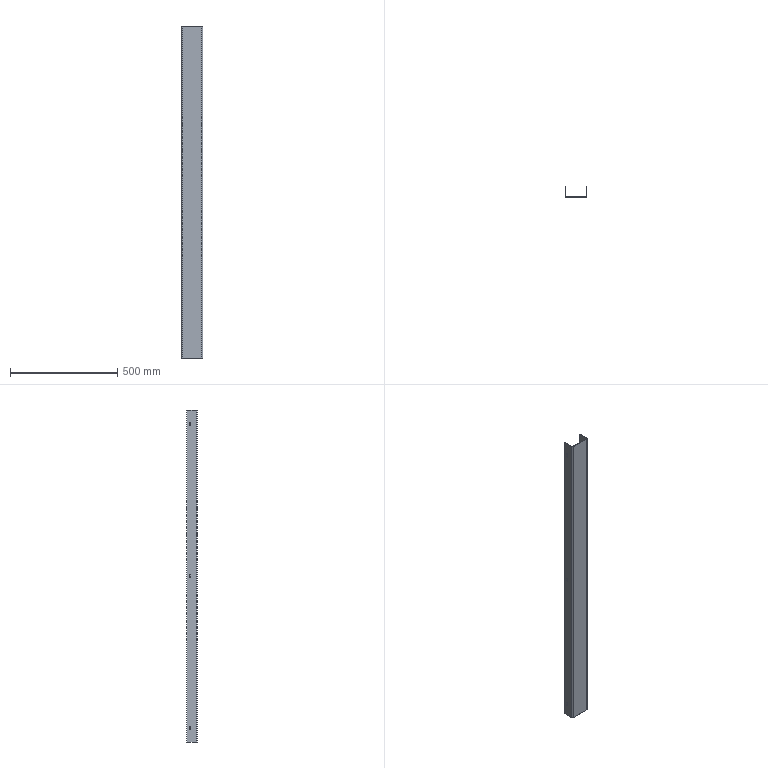Part | SolidWorks | features ICE 2, LPattern 2, FlatPattern 1, SMBaseFlange 1, SheetMetal 1 | 1 solid | 43 faces | box 100 x 50 x 1550 mm | volume 886864 mm3 | plane 24 | cylinder 19 | commonest cylinder face diameters 7 x9 6.4 x6 4 x2 10 x2
STEP:
#1=CARTESIAN_POINT('',(149.265,50.375,780.));
#2=VERTEX_POINT('',#1);
#3=CARTESIAN_POINT('',(149.265,46.875,783.5));
#4=VERTEX_POINT('',#3);
#5=CARTESIAN_POINT('',(149.265,46.875,780.));
#6=DIRECTION('',(1.,0.,0.));
#7=DIRECTION('',(0.,0.,-1.));
#8=AXIS2_PLACEMENT_3D('',#5,#6,#7);
#9=CIRCLE('',#8,3.5);
#10=EDGE_CURVE('',#2,#4,#9,.T.);
#11=ORIENTED_EDGE('',*,*,#10,.T.);
#12=CARTESIAN_POINT('',(146.265,46.875,783.5));
#13=VERTEX_POINT('',#12);
#14=CARTESIAN_POINT('',(156.265,46.875,783.5));
#15=DIRECTION('',(-1.,0.,0.));
#16=VECTOR('',#15,1000.);
#17=LINE('',#14,#16);
#18=EDGE_CURVE('',#4,#13,#17,.T.);
#19=ORIENTED_EDGE('',*,*,#18,.T.);
#20=CARTESIAN_POINT('',(146.265,50.375,780.));
#21=VERTEX_POINT('',#20);
#22=CARTESIAN_POINT('',(146.265,46.875,780.));
#23=DIRECTION('',(-1.,0.,0.));
#24=DIRECTION('',(0.,0.,1.));
#25=AXIS2_PLACEMENT_3D('',#22,#23,#24);
#26=CIRCLE('',#25,3.5);
#27=EDGE_CURVE('',#13,#21,#26,.T.);
#28=ORIENTED_EDGE('',*,*,#27,.T.);
#29=CARTESIAN_POINT('',(156.265,50.375,780.));
#30=DIRECTION('',(-1.,0.,0.));
#31=VECTOR('',#30,1000.);
#32=LINE('',#29,#31);
#33=EDGE_CURVE('',#2,#21,#32,.T.);
#34=ORIENTED_EDGE('',*,*,#33,.F.);
#35=EDGE_LOOP('',(#11,#19,#28,#34));
#36=FACE_OUTER_BOUND('',#35,.T.);
#37=CARTESIAN_POINT('',(156.265,46.875,780.));
#38=DIRECTION('',(-1.,0.,0.));
#39=DIRECTION('',(0.,0.,1.));
#40=AXIS2_PLACEMENT_3D('',#37,#38,#39);
#41=CYLINDRICAL_SURFACE('',#40,3.5);
#42=ADVANCED_FACE('',(#36),#41,.F.);
#43=CARTESIAN_POINT('',(149.265,50.375,70.));
#44=VERTEX_POINT('',#43);
#45=CARTESIAN_POINT('',(149.265,46.875,73.5));
#46=VERTEX_POINT('',#45);
#47=CARTESIAN_POINT('',(149.265,46.875,70.));
#48=DIRECTION('',(1.,0.,0.));
#49=DIRECTION('',(0.,0.,-1.));
#50=AXIS2_PLACEMENT_3D('',#47,#48,#49);
#51=CIRCLE('',#50,3.5);
#52=EDGE_CURVE('',#44,#46,#51,.T.);
#53=ORIENTED_EDGE('',*,*,#52,.T.);
#54=CARTESIAN_POINT('',(146.265,46.875,73.5));
#55=VERTEX_POINT('',#54);
#56=CARTESIAN_POINT('',(156.265,46.875,73.5));
#57=DIRECTION('',(-1.,0.,0.));
#58=VECTOR('',#57,1000.);
#59=LINE('',#56,#58);
#60=EDGE_CURVE('',#46,#55,#59,.T.);
#61=ORIENTED_EDGE('',*,*,#60,.T.);
#62=CARTESIAN_POINT('',(146.265,50.375,70.));
#63=VERTEX_POINT('',#62);
#64=CARTESIAN_POINT('',(146.265,46.875,70.));
#65=DIRECTION('',(-1.,0.,0.));
#66=DIRECTION('',(0.,0.,1.));
#67=AXIS2_PLACEMENT_3D('',#64,#65,#66);
#68=CIRCLE('',#67,3.5);
#69=EDGE_CURVE('',#55,#63,#68,.T.);
#70=ORIENTED_EDGE('',*,*,#69,.T.);
#71=CARTESIAN_POINT('',(156.265,50.375,70.));
#72=DIRECTION('',(-1.,0.,0.));
#73=VECTOR('',#72,1000.);
#74=LINE('',#71,#73);
#75=EDGE_CURVE('',#44,#63,#74,.T.);
#76=ORIENTED_EDGE('',*,*,#75,.F.);
#77=EDGE_LOOP('',(#53,#61,#70,#76));
#78=FACE_OUTER_BOUND('',#77,.T.);
#79=CARTESIAN_POINT('',(156.265,46.875,70.));
#80=DIRECTION('',(-1.,0.,0.));
#81=DIRECTION('',(0.,0.,1.));
#82=AXIS2_PLACEMENT_3D('',#79,#80,#81);
#83=CYLINDRICAL_SURFACE('',#82,3.5);
#84=ADVANCED_FACE('',(#78),#83,.F.);
#85=CARTESIAN_POINT('',(243.265,51.875,771.8));
#86=VERTEX_POINT('',#85);
#87=CARTESIAN_POINT('',(243.265,51.875,778.2));
#88=VERTEX_POINT('',#87);
#89=CARTESIAN_POINT('',(243.265,51.875,775.));
#90=DIRECTION('',(-1.,0.,0.));
#91=DIRECTION('',(0.,0.,1.));
#92=AXIS2_PLACEMENT_3D('',#89,#90,#91);
#93=CIRCLE('',#92,3.2);
#94=EDGE_CURVE('',#86,#88,#93,.T.);
#95=ORIENTED_EDGE('',*,*,#94,.T.);
#96=CARTESIAN_POINT('',(246.265,51.875,778.2));
#97=VERTEX_POINT('',#96);
#98=CARTESIAN_POINT('',(236.265,51.875,778.2));
#99=DIRECTION('',(1.,0.,0.));
#100=VECTOR('',#99,1000.);
#101=LINE('',#98,#100);
#102=EDGE_CURVE('',#88,#97,#101,.T.);
#103=ORIENTED_EDGE('',*,*,#102,.T.);
#104=CARTESIAN_POINT('',(246.265,51.875,771.8));
#105=VERTEX_POINT('',#104);
#106=CARTESIAN_POINT('',(246.265,51.875,775.));
#107=DIRECTION('',(1.,0.,0.));
#108=DIRECTION('',(0.,0.,-1.));
#109=AXIS2_PLACEMENT_3D('',#106,#107,#108);
#110=CIRCLE('',#109,3.2);
#111=EDGE_CURVE('',#97,#105,#110,.T.);
#112=ORIENTED_EDGE('',*,*,#111,.T.);
#113=CARTESIAN_POINT('',(236.265,51.875,771.8));
#114=DIRECTION('',(1.,0.,0.));
#115=VECTOR('',#114,1000.);
#116=LINE('',#113,#115);
#117=EDGE_CURVE('',#86,#105,#116,.T.);
#118=ORIENTED_EDGE('',*,*,#117,.F.);
#119=EDGE_LOOP('',(#95,#103,#112,#118));
#120=FACE_OUTER_BOUND('',#119,.T.);
#121=CARTESIAN_POINT('',(236.265,51.875,775.));
#122=DIRECTION('',(1.,0.,0.));
#123=DIRECTION('',(0.,0.,-1.));
#124=AXIS2_PLACEMENT_3D('',#121,#122,#123);
#125=CYLINDRICAL_SURFACE('',#124,3.2);
#126=ADVANCED_FACE('',(#120),#125,.F.);
#127=CARTESIAN_POINT('',(243.265,51.875,1484.3));
#128=VERTEX_POINT('',#127);
#129=CARTESIAN_POINT('',(243.265,51.875,1490.7));
#130=VERTEX_POINT('',#129);
#131=CARTESIAN_POINT('',(243.265,51.875,1487.5));
#132=DIRECTION('',(-1.,0.,0.));
#133=DIRECTION('',(0.,0.,1.));
#134=AXIS2_PLACEMENT_3D('',#131,#132,#133);
#135=CIRCLE('',#134,3.2);
#136=EDGE_CURVE('',#128,#130,#135,.T.);
#137=ORIENTED_EDGE('',*,*,#136,.T.);
#138=CARTESIAN_POINT('',(246.265,51.875,1490.7));
#139=VERTEX_POINT('',#138);
#140=CARTESIAN_POINT('',(236.265,51.875,1490.7));
#141=DIRECTION('',(1.,0.,0.));
#142=VECTOR('',#141,1000.);
#143=LINE('',#140,#142);
#144=EDGE_CURVE('',#130,#139,#143,.T.);
#145=ORIENTED_EDGE('',*,*,#144,.T.);
#146=CARTESIAN_POINT('',(246.265,51.875,1484.3));
#147=VERTEX_POINT('',#146);
#148=CARTESIAN_POINT('',(246.265,51.875,1487.5));
#149=DIRECTION('',(1.,0.,0.));
#150=DIRECTION('',(0.,0.,-1.));
#151=AXIS2_PLACEMENT_3D('',#148,#149,#150);
#152=CIRCLE('',#151,3.2);
#153=EDGE_CURVE('',#139,#147,#152,.T.);
#154=ORIENTED_EDGE('',*,*,#153,.T.);
#155=CARTESIAN_POINT('',(236.265,51.875,1484.3));
#156=DIRECTION('',(1.,0.,0.));
#157=VECTOR('',#156,1000.);
#158=LINE('',#155,#157);
#159=EDGE_CURVE('',#128,#147,#158,.T.);
#160=ORIENTED_EDGE('',*,*,#159,.F.);
#161=EDGE_LOOP('',(#137,#145,#154,#160));
#162=FACE_OUTER_BOUND('',#161,.T.);
#163=CARTESIAN_POINT('',(236.265,51.875,1487.5));
#164=DIRECTION('',(1.,0.,0.));
#165=DIRECTION('',(0.,0.,-1.));
#166=AXIS2_PLACEMENT_3D('',#163,#164,#165);
#167=CYLINDRICAL_SURFACE('',#166,3.2);
#168=ADVANCED_FACE('',(#162),#167,.F.);
#169=CARTESIAN_POINT('',(243.265,51.875,59.3));
#170=VERTEX_POINT('',#169);
#171=CARTESIAN_POINT('',(243.265,51.875,65.7));
#172=VERTEX_POINT('',#171);
#173=CARTESIAN_POINT('',(243.265,51.875,62.5));
#174=DIRECTION('',(-1.,0.,0.));
#175=DIRECTION('',(0.,0.,1.));
#176=AXIS2_PLACEMENT_3D('',#173,#174,#175);
#177=CIRCLE('',#176,3.2);
#178=EDGE_CURVE('',#170,#172,#177,.T.);
#179=ORIENTED_EDGE('',*,*,#178,.T.);
#180=CARTESIAN_POINT('',(246.265,51.875,65.7));
#181=VERTEX_POINT('',#180);
#182=CARTESIAN_POINT('',(236.265,51.875,65.7));
#183=DIRECTION('',(1.,0.,0.));
#184=VECTOR('',#183,1000.);
#185=LINE('',#182,#184);
#186=EDGE_CURVE('',#172,#181,#185,.T.);
#187=ORIENTED_EDGE('',*,*,#186,.T.);
#188=CARTESIAN_POINT('',(246.265,51.875,59.3));
#189=VERTEX_POINT('',#188);
#190=CARTESIAN_POINT('',(246.265,51.875,62.5));
#191=DIRECTION('',(1.,0.,0.));
#192=DIRECTION('',(0.,0.,-1.));
#193=AXIS2_PLACEMENT_3D('',#190,#191,#192);
#194=CIRCLE('',#193,3.2);
#195=EDGE_CURVE('',#181,#189,#194,.T.);
#196=ORIENTED_EDGE('',*,*,#195,.T.);
#197=CARTESIAN_POINT('',(236.265,51.875,59.3));
#198=DIRECTION('',(1.,0.,0.));
#199=VECTOR('',#198,1000.);
#200=LINE('',#197,#199);
#201=EDGE_CURVE('',#170,#189,#200,.T.);
#202=ORIENTED_EDGE('',*,*,#201,.F.);
#203=EDGE_LOOP('',(#179,#187,#196,#202));
#204=FACE_OUTER_BOUND('',#203,.T.);
#205=CARTESIAN_POINT('',(236.265,51.875,62.5));
#206=DIRECTION('',(1.,0.,0.));
#207=DIRECTION('',(0.,0.,-1.));
#208=AXIS2_PLACEMENT_3D('',#205,#206,#207);
#209=CYLINDRICAL_SURFACE('',#208,3.2);
#210=ADVANCED_FACE('',(#204),#209,.F.);
#211=CARTESIAN_POINT('',(149.265,50.375,1490.));
#212=VERTEX_POINT('',#211);
#213=CARTESIAN_POINT('',(149.265,46.875,1493.5));
#214=VERTEX_POINT('',#213);
#215=CARTESIAN_POINT('',(149.265,46.875,1490.));
#216=DIRECTION('',(1.,0.,0.));
#217=DIRECTION('',(0.,0.,-1.));
#218=AXIS2_PLACEMENT_3D('',#215,#216,#217);
#219=CIRCLE('',#218,3.5);
#220=EDGE_CURVE('',#212,#214,#219,.T.);
#221=ORIENTED_EDGE('',*,*,#220,.T.);
#222=CARTESIAN_POINT('',(146.265,46.875,1493.5));
#223=VERTEX_POINT('',#222);
#224=CARTESIAN_POINT('',(156.265,46.875,1493.5));
#225=DIRECTION('',(-1.,0.,0.));
#226=VECTOR('',#225,1000.);
#227=LINE('',#224,#226);
#228=EDGE_CURVE('',#214,#223,#227,.T.);
#229=ORIENTED_EDGE('',*,*,#228,.T.);
#230=CARTESIAN_POINT('',(146.265,50.375,1490.));
#231=VERTEX_POINT('',#230);
#232=CARTESIAN_POINT('',(146.265,46.875,1490.));
#233=DIRECTION('',(-1.,0.,0.));
#234=DIRECTION('',(0.,0.,1.));
#235=AXIS2_PLACEMENT_3D('',#232,#233,#234);
#236=CIRCLE('',#235,3.5);
#237=EDGE_CURVE('',#223,#231,#236,.T.);
#238=ORIENTED_EDGE('',*,*,#237,.T.);
#239=CARTESIAN_POINT('',(156.265,50.375,1490.));
#240=DIRECTION('',(-1.,0.,0.));
#241=VECTOR('',#240,1000.);
#242=LINE('',#239,#241);
#243=EDGE_CURVE('',#212,#231,#242,.T.);
#244=ORIENTED_EDGE('',*,*,#243,.F.);
#245=EDGE_LOOP('',(#221,#229,#238,#244));
#246=FACE_OUTER_BOUND('',#245,.T.);
#247=CARTESIAN_POINT('',(156.265,46.875,1490.));
#248=DIRECTION('',(-1.,0.,0.));
#249=DIRECTION('',(0.,0.,1.));
#250=AXIS2_PLACEMENT_3D('',#247,#248,#249);
#251=CYLINDRICAL_SURFACE('',#250,3.5);
#252=ADVANCED_FACE('',(#246),#251,.F.);
#253=CARTESIAN_POINT('',(149.265,43.375,1490.));
#254=VERTEX_POINT('',#253);
#255=CARTESIAN_POINT('',(149.265,43.375,1480.));
#256=VERTEX_POINT('',#255);
#257=CARTESIAN_POINT('',(149.265,43.375,2970.));
#258=DIRECTION('',(0.,0.,-1.));
#259=VECTOR('',#258,1000.);
#260=LINE('',#257,#259);
#261=EDGE_CURVE('',#254,#256,#260,.T.);
#262=ORIENTED_EDGE('',*,*,#261,.T.);
#263=CARTESIAN_POINT('',(146.265,43.375,1480.));
#264=VERTEX_POINT('',#263);
#265=CARTESIAN_POINT('',(156.265,43.375,1480.));
#266=DIRECTION('',(-1.,0.,0.));
#267=VECTOR('',#266,1000.);
#268=LINE('',#265,#267);
#269=EDGE_CURVE('',#256,#264,#268,.T.);
#270=ORIENTED_EDGE('',*,*,#269,.T.);
#271=CARTESIAN_POINT('',(146.265,43.375,1490.));
#272=VERTEX_POINT('',#271);
#273=CARTESIAN_POINT('',(146.265,43.375,1480.));
#274=DIRECTION('',(0.,0.,1.));
#275=VECTOR('',#274,1000.);
#276=LINE('',#273,#275);
#277=EDGE_CURVE('',#264,#272,#276,.T.);
#278=ORIENTED_EDGE('',*,*,#277,.T.);
#279=CARTESIAN_POINT('',(156.265,43.375,1490.));
#280=DIRECTION('',(-1.,0.,0.));
#281=VECTOR('',#280,1000.);
#282=LINE('',#279,#281);
#283=EDGE_CURVE('',#254,#272,#282,.T.);
#284=ORIENTED_EDGE('',*,*,#283,.F.);
#285=EDGE_LOOP('',(#262,#270,#278,#284));
#286=FACE_OUTER_BOUND('',#285,.T.);
#287=CARTESIAN_POINT('',(156.265,43.375,1480.));
#288=DIRECTION('',(0.,-1.,0.));
#289=DIRECTION('',(0.,0.,-1.));
#290=AXIS2_PLACEMENT_3D('',#287,#288,#289);
#291=PLANE('',#290);
#292=ADVANCED_FACE('',(#286),#291,.F.);
#293=ORIENTED_EDGE('',*,*,#228,.F.);
#294=CARTESIAN_POINT('',(149.265,46.875,1490.));
#295=DIRECTION('',(1.,0.,0.));
#296=DIRECTION('',(0.,0.,-1.));
#297=AXIS2_PLACEMENT_3D('',#294,#295,#296);
#298=CIRCLE('',#297,3.5);
#299=EDGE_CURVE('',#214,#254,#298,.T.);
#300=ORIENTED_EDGE('',*,*,#299,.T.);
#301=ORIENTED_EDGE('',*,*,#283,.T.);
#302=CARTESIAN_POINT('',(146.265,46.875,1490.));
#303=DIRECTION('',(-1.,0.,0.));
#304=DIRECTION('',(0.,0.,1.));
#305=AXIS2_PLACEMENT_3D('',#302,#303,#304);
#306=CIRCLE('',#305,3.5);
#307=EDGE_CURVE('',#272,#223,#306,.T.);
#308=ORIENTED_EDGE('',*,*,#307,.T.);
#309=EDGE_LOOP('',(#293,#300,#301,#308));
#310=FACE_OUTER_BOUND('',#309,.T.);
#311=CARTESIAN_POINT('',(156.265,46.875,1490.));
#312=DIRECTION('',(-1.,0.,0.));
#313=DIRECTION('',(0.,0.,1.));
#314=AXIS2_PLACEMENT_3D('',#311,#312,#313);
#315=CYLINDRICAL_SURFACE('',#314,3.5);
#316=ADVANCED_FACE('',(#310),#315,.F.);
#317=CARTESIAN_POINT('',(149.265,50.375,1480.));
#318=VERTEX_POINT('',#317);
#319=CARTESIAN_POINT('',(149.265,50.375,2970.));
#320=DIRECTION('',(0.,0.,1.));
#321=VECTOR('',#320,1000.);
#322=LINE('',#319,#321);
#323=EDGE_CURVE('',#318,#212,#322,.T.);
#324=ORIENTED_EDGE('',*,*,#323,.T.);
#325=ORIENTED_EDGE('',*,*,#243,.T.);
#326=CARTESIAN_POINT('',(146.265,50.375,1480.));
#327=VERTEX_POINT('',#326);
#328=CARTESIAN_POINT('',(146.265,50.375,1480.));
#329=DIRECTION('',(0.,0.,-1.));
#330=VECTOR('',#329,1000.);
#331=LINE('',#328,#330);
#332=EDGE_CURVE('',#231,#327,#331,.T.);
#333=ORIENTED_EDGE('',*,*,#332,.T.);
#334=CARTESIAN_POINT('',(156.265,50.375,1480.));
#335=DIRECTION('',(-1.,0.,0.));
#336=VECTOR('',#335,1000.);
#337=LINE('',#334,#336);
#338=EDGE_CURVE('',#318,#327,#337,.T.);
#339=ORIENTED_EDGE('',*,*,#338,.F.);
#340=EDGE_LOOP('',(#324,#325,#333,#339));
#341=FACE_OUTER_BOUND('',#340,.T.);
#342=CARTESIAN_POINT('',(156.265,50.375,1480.));
#343=DIRECTION('',(0.,1.,0.));
#344=DIRECTION('',(0.,0.,1.));
#345=AXIS2_PLACEMENT_3D('',#342,#343,#344);
#346=PLANE('',#345);
#347=ADVANCED_FACE('',(#341),#346,.F.);
#348=CARTESIAN_POINT('',(149.265,46.875,1480.));
#349=DIRECTION('',(1.,0.,0.));
#350=DIRECTION('',(0.,0.,-1.));
#351=AXIS2_PLACEMENT_3D('',#348,#349,#350);
#352=CIRCLE('',#351,3.5);
#353=EDGE_CURVE('',#256,#318,#352,.T.);
#354=ORIENTED_EDGE('',*,*,#353,.T.);
#355=ORIENTED_EDGE('',*,*,#338,.T.);
#356=CARTESIAN_POINT('',(146.265,46.875,1480.));
#357=DIRECTION('',(-1.,0.,0.));
#358=DIRECTION('',(0.,0.,1.));
#359=AXIS2_PLACEMENT_3D('',#356,#357,#358);
#360=CIRCLE('',#359,3.5);
#361=EDGE_CURVE('',#327,#264,#360,.T.);
#362=ORIENTED_EDGE('',*,*,#361,.T.);
#363=ORIENTED_EDGE('',*,*,#269,.F.);
#364=EDGE_LOOP('',(#354,#355,#362,#363));
#365=FACE_OUTER_BOUND('',#364,.T.);
#366=CARTESIAN_POINT('',(156.265,46.875,1480.));
#367=DIRECTION('',(-1.,0.,0.));
#368=DIRECTION('',(0.,0.,1.));
#369=AXIS2_PLACEMENT_3D('',#366,#367,#368);
#370=CYLINDRICAL_SURFACE('',#369,3.5);
#371=ADVANCED_FACE('',(#365),#370,.F.);
#372=ORIENTED_EDGE('',*,*,#186,.F.);
#373=CARTESIAN_POINT('',(243.265,51.875,62.5));
#374=DIRECTION('',(-1.,0.,0.));
#375=DIRECTION('',(0.,0.,1.));
#376=AXIS2_PLACEMENT_3D('',#373,#374,#375);
#377=CIRCLE('',#376,3.2);
#378=EDGE_CURVE('',#172,#170,#377,.T.);
#379=ORIENTED_EDGE('',*,*,#378,.T.);
#380=ORIENTED_EDGE('',*,*,#201,.T.);
#381=CARTESIAN_POINT('',(246.265,51.875,62.5));
#382=DIRECTION('',(1.,0.,0.));
#383=DIRECTION('',(0.,0.,-1.));
#384=AXIS2_PLACEMENT_3D('',#381,#382,#383);
#385=CIRCLE('',#384,3.2);
#386=EDGE_CURVE('',#189,#181,#385,.T.);
#387=ORIENTED_EDGE('',*,*,#386,.T.);
#388=EDGE_LOOP('',(#372,#379,#380,#387));
#389=FACE_OUTER_BOUND('',#388,.T.);
#390=CARTESIAN_POINT('',(236.265,51.875,62.5));
#391=DIRECTION('',(1.,0.,0.));
#392=DIRECTION('',(0.,0.,-1.));
#393=AXIS2_PLACEMENT_3D('',#390,#391,#392);
#394=CYLINDRICAL_SURFACE('',#393,3.2);
#395=ADVANCED_FACE('',(#389),#394,.F.);
#396=CARTESIAN_POINT('',(146.265,16.875,1550.));
#397=VERTEX_POINT('',#396);
#398=CARTESIAN_POINT('',(149.265,16.875,1550.));
#399=VERTEX_POINT('',#398);
#400=CARTESIAN_POINT('',(146.265,16.875,1550.));
#401=DIRECTION('',(1.,0.,0.));
#402=VECTOR('',#401,1000.);
#403=LINE('',#400,#402);
#404=EDGE_CURVE('',#397,#399,#403,.T.);
#405=ORIENTED_EDGE('',*,*,#404,.F.);
#406=CARTESIAN_POINT('',(151.265,11.875,1550.));
#407=VERTEX_POINT('',#406);
#408=CARTESIAN_POINT('',(151.265,16.875,1550.));
#409=DIRECTION('',(0.,0.,1.));
#410=DIRECTION('',(-1.,0.,0.));
#411=AXIS2_PLACEMENT_3D('',#408,#409,#410);
#412=CIRCLE('',#411,5.);
#413=EDGE_CURVE('',#397,#407,#412,.T.);
#414=ORIENTED_EDGE('',*,*,#413,.T.);
#415=CARTESIAN_POINT('',(151.265,14.875,1550.));
#416=VERTEX_POINT('',#415);
#417=CARTESIAN_POINT('',(151.265,14.875,1550.));
#418=DIRECTION('',(0.,-1.,0.));
#419=VECTOR('',#418,1000.);
#420=LINE('',#417,#419);
#421=EDGE_CURVE('',#416,#407,#420,.T.);
#422=ORIENTED_EDGE('',*,*,#421,.F.);
#423=CARTESIAN_POINT('',(151.265,16.875,1550.));
#424=DIRECTION('',(0.,0.,1.));
#425=DIRECTION('',(1.,0.,0.));
#426=AXIS2_PLACEMENT_3D('',#423,#424,#425);
#427=CIRCLE('',#426,2.);
#428=EDGE_CURVE('',#399,#416,#427,.T.);
#429=ORIENTED_EDGE('',*,*,#428,.F.);
#430=EDGE_LOOP('',(#405,#414,#422,#429));
#431=FACE_OUTER_BOUND('',#430,.T.);
#432=CARTESIAN_POINT('',(146.265,16.875,1550.));
#433=DIRECTION('',(0.,0.,1.));
#434=DIRECTION('',(1.,0.,0.));
#435=AXIS2_PLACEMENT_3D('',#432,#433,#434);
#436=PLANE('',#435);
#437=ADVANCED_FACE('',(#431),#436,.T.);
#438=CARTESIAN_POINT('',(146.265,61.875,1550.));
#439=VERTEX_POINT('',#438);
#440=CARTESIAN_POINT('',(146.265,61.875,1550.));
#441=DIRECTION('',(0.,-1.,0.));
#442=VECTOR('',#441,1000.);
#443=LINE('',#440,#442);
#444=EDGE_CURVE('',#439,#397,#443,.T.);
#445=ORIENTED_EDGE('',*,*,#444,.T.);
#446=ORIENTED_EDGE('',*,*,#404,.T.);
#447=CARTESIAN_POINT('',(149.265,61.875,1550.));
#448=VERTEX_POINT('',#447);
#449=CARTESIAN_POINT('',(149.265,61.875,1550.));
#450=DIRECTION('',(0.,-1.,0.));
#451=VECTOR('',#450,1000.);
#452=LINE('',#449,#451);
#453=EDGE_CURVE('',#448,#399,#452,.T.);
#454=ORIENTED_EDGE('',*,*,#453,.F.);
#455=CARTESIAN_POINT('',(146.265,61.875,1550.));
#456=DIRECTION('',(1.,0.,0.));
#457=VECTOR('',#456,1000.);
#458=LINE('',#455,#457);
#459=EDGE_CURVE('',#439,#448,#458,.T.);
#460=ORIENTED_EDGE('',*,*,#459,.F.);
#461=EDGE_LOOP('',(#445,#446,#454,#460));
#462=FACE_OUTER_BOUND('',#461,.T.);
#463=CARTESIAN_POINT('',(151.265,14.875,1550.));
#464=DIRECTION('',(0.,0.,1.));
#465=DIRECTION('',(1.,0.,0.));
#466=AXIS2_PLACEMENT_3D('',#463,#464,#465);
#467=PLANE('',#466);
#468=ADVANCED_FACE('',(#462),#467,.T.);
#469=CARTESIAN_POINT('',(151.265,11.875,0.));
#470=VERTEX_POINT('',#469);
#471=CARTESIAN_POINT('',(151.265,14.875,0.));
#472=VERTEX_POINT('',#471);
#473=CARTESIAN_POINT('',(151.265,11.875,0.));
#474=DIRECTION('',(0.,1.,0.));
#475=VECTOR('',#474,1000.);
#476=LINE('',#473,#475);
#477=EDGE_CURVE('',#470,#472,#476,.T.);
#478=ORIENTED_EDGE('',*,*,#477,.F.);
#479=CARTESIAN_POINT('',(146.265,16.875,0.));
#480=VERTEX_POINT('',#479);
#481=CARTESIAN_POINT('',(151.265,16.875,0.));
#482=DIRECTION('',(0.,0.,1.));
#483=DIRECTION('',(-1.,0.,0.));
#484=AXIS2_PLACEMENT_3D('',#481,#482,#483);
#485=CIRCLE('',#484,5.);
#486=EDGE_CURVE('',#480,#470,#485,.T.);
#487=ORIENTED_EDGE('',*,*,#486,.F.);
#488=CARTESIAN_POINT('',(149.265,16.875,0.));
#489=VERTEX_POINT('',#488);
#490=CARTESIAN_POINT('',(149.265,16.875,0.));
#491=DIRECTION('',(-1.,0.,0.));
#492=VECTOR('',#491,1000.);
#493=LINE('',#490,#492);
#494=EDGE_CURVE('',#489,#480,#493,.T.);
#495=ORIENTED_EDGE('',*,*,#494,.F.);
#496=CARTESIAN_POINT('',(151.265,16.875,0.));
#497=DIRECTION('',(0.,0.,1.));
#498=DIRECTION('',(1.,0.,0.));
#499=AXIS2_PLACEMENT_3D('',#496,#497,#498);
#500=CIRCLE('',#499,2.);
#501=EDGE_CURVE('',#489,#472,#500,.T.);
#502=ORIENTED_EDGE('',*,*,#501,.T.);
#503=EDGE_LOOP('',(#478,#487,#495,#502));
#504=FACE_OUTER_BOUND('',#503,.T.);
#505=CARTESIAN_POINT('',(151.265,11.875,0.));
#506=DIRECTION('',(0.,0.,-1.));
#507=DIRECTION('',(-1.,0.,0.));
#508=AXIS2_PLACEMENT_3D('',#505,#506,#507);
#509=PLANE('',#508);
#510=ADVANCED_FACE('',(#504),#509,.T.);
#511=CARTESIAN_POINT('',(241.265,11.875,0.));
#512=VERTEX_POINT('',#511);
#513=CARTESIAN_POINT('',(146.265,11.875,0.));
#514=DIRECTION('',(1.,0.,0.));
#515=VECTOR('',#514,1000.);
#516=LINE('',#513,#515);
#517=EDGE_CURVE('',#470,#512,#516,.T.);
#518=ORIENTED_EDGE('',*,*,#517,.F.);
#519=ORIENTED_EDGE('',*,*,#477,.T.);
#520=CARTESIAN_POINT('',(241.265,14.875,0.));
#521=VERTEX_POINT('',#520);
#522=CARTESIAN_POINT('',(146.265,14.875,0.));
#523=DIRECTION('',(1.,0.,0.));
#524=VECTOR('',#523,1000.);
#525=LINE('',#522,#524);
#526=EDGE_CURVE('',#472,#521,#525,.T.);
#527=ORIENTED_EDGE('',*,*,#526,.T.);
#528=CARTESIAN_POINT('',(241.265,14.875,0.));
#529=DIRECTION('',(0.,-1.,0.));
#530=VECTOR('',#529,1000.);
#531=LINE('',#528,#530);
#532=EDGE_CURVE('',#521,#512,#531,.T.);
#533=ORIENTED_EDGE('',*,*,#532,.T.);
#534=EDGE_LOOP('',(#518,#519,#527,#533));
#535=FACE_OUTER_BOUND('',#534,.T.);
#536=CARTESIAN_POINT('',(149.265,16.875,0.));
#537=DIRECTION('',(0.,0.,-1.));
#538=DIRECTION('',(-1.,0.,0.));
#539=AXIS2_PLACEMENT_3D('',#536,#537,#538);
#540=PLANE('',#539);
#541=ADVANCED_FACE('',(#535),#540,.T.);
#542=CARTESIAN_POINT('',(241.265,11.875,1550.));
#543=VERTEX_POINT('',#542);
#544=CARTESIAN_POINT('',(241.265,14.875,1550.));
#545=VERTEX_POINT('',#544);
#546=CARTESIAN_POINT('',(241.265,11.875,1550.));
#547=DIRECTION('',(0.,1.,0.));
#548=VECTOR('',#547,1000.);
#549=LINE('',#546,#548);
#550=EDGE_CURVE('',#543,#545,#549,.T.);
#551=ORIENTED_EDGE('',*,*,#550,.F.);
#552=CARTESIAN_POINT('',(246.265,16.875,1550.));
#553=VERTEX_POINT('',#552);
#554=CARTESIAN_POINT('',(241.265,16.875,1550.));
#555=DIRECTION('',(0.,0.,1.));
#556=DIRECTION('',(-1.,0.,0.));
#557=AXIS2_PLACEMENT_3D('',#554,#555,#556);
#558=CIRCLE('',#557,5.);
#559=EDGE_CURVE('',#543,#553,#558,.T.);
#560=ORIENTED_EDGE('',*,*,#559,.T.);
#561=CARTESIAN_POINT('',(243.265,16.875,1550.));
#562=VERTEX_POINT('',#561);
#563=CARTESIAN_POINT('',(243.265,16.875,1550.));
#564=DIRECTION('',(1.,0.,0.));
#565=VECTOR('',#564,1000.);
#566=LINE('',#563,#565);
#567=EDGE_CURVE('',#562,#553,#566,.T.);
#568=ORIENTED_EDGE('',*,*,#567,.F.);
#569=CARTESIAN_POINT('',(241.265,16.875,1550.));
#570=DIRECTION('',(0.,0.,1.));
#571=DIRECTION('',(1.,0.,0.));
#572=AXIS2_PLACEMENT_3D('',#569,#570,#571);
#573=CIRCLE('',#572,2.);
#574=EDGE_CURVE('',#545,#562,#573,.T.);
#575=ORIENTED_EDGE('',*,*,#574,.F.);
#576=EDGE_LOOP('',(#551,#560,#568,#575));
#577=FACE_OUTER_BOUND('',#576,.T.);
#578=CARTESIAN_POINT('',(241.265,11.875,1550.));
#579=DIRECTION('',(0.,0.,1.));
#580=DIRECTION('',(1.,0.,0.));
#581=AXIS2_PLACEMENT_3D('',#578,#579,#580);
#582=PLANE('',#581);
#583=ADVANCED_FACE('',(#577),#582,.T.);
#584=CARTESIAN_POINT('',(146.265,11.875,1550.));
#585=DIRECTION('',(1.,0.,0.));
#586=VECTOR('',#585,1000.);
#587=LINE('',#584,#586);
#588=EDGE_CURVE('',#407,#543,#587,.T.);
#589=ORIENTED_EDGE('',*,*,#588,.T.);
#590=ORIENTED_EDGE('',*,*,#550,.T.);
#591=CARTESIAN_POINT('',(146.265,14.875,1550.));
#592=DIRECTION('',(1.,0.,0.));
#593=VECTOR('',#592,1000.);
#594=LINE('',#591,#593);
#595=EDGE_CURVE('',#416,#545,#594,.T.);
#596=ORIENTED_EDGE('',*,*,#595,.F.);
#597=ORIENTED_EDGE('',*,*,#421,.T.);
#598=EDGE_LOOP('',(#589,#590,#596,#597));
#599=FACE_OUTER_BOUND('',#598,.T.);
#600=CARTESIAN_POINT('',(243.265,16.875,1550.));
#601=DIRECTION('',(0.,0.,1.));
#602=DIRECTION('',(1.,0.,0.));
#603=AXIS2_PLACEMENT_3D('',#600,#601,#602);
#604=PLANE('',#603);
#605=ADVANCED_FACE('',(#599),#604,.T.);
#606=CARTESIAN_POINT('',(246.265,16.875,0.));
#607=VERTEX_POINT('',#606);
#608=CARTESIAN_POINT('',(243.265,16.875,0.));
#609=VERTEX_POINT('',#608);
#610=CARTESIAN_POINT('',(246.265,16.875,0.));
#611=DIRECTION('',(-1.,0.,0.));
#612=VECTOR('',#611,1000.);
#613=LINE('',#610,#612);
#614=EDGE_CURVE('',#607,#609,#613,.T.);
#615=ORIENTED_EDGE('',*,*,#614,.F.);
#616=CARTESIAN_POINT('',(241.265,16.875,0.));
#617=DIRECTION('',(0.,0.,1.));
#618=DIRECTION('',(-1.,0.,0.));
#619=AXIS2_PLACEMENT_3D('',#616,#617,#618);
#620=CIRCLE('',#619,5.);
#621=EDGE_CURVE('',#512,#607,#620,.T.);
#622=ORIENTED_EDGE('',*,*,#621,.F.);
#623=ORIENTED_EDGE('',*,*,#532,.F.);
#624=CARTESIAN_POINT('',(241.265,16.875,0.));
#625=DIRECTION('',(0.,0.,1.));
#626=DIRECTION('',(1.,0.,0.));
#627=AXIS2_PLACEMENT_3D('',#624,#625,#626);
#628=CIRCLE('',#627,2.);
#629=EDGE_CURVE('',#521,#609,#628,.T.);
#630=ORIENTED_EDGE('',*,*,#629,.T.);
#631=EDGE_LOOP('',(#615,#622,#623,#630));
#632=FACE_OUTER_BOUND('',#631,.T.);
#633=CARTESIAN_POINT('',(246.265,16.875,0.));
#634=DIRECTION('',(0.,0.,-1.));
#635=DIRECTION('',(-1.,0.,0.));
#636=AXIS2_PLACEMENT_3D('',#633,#634,#635);
#637=PLANE('',#636);
#638=ADVANCED_FACE('',(#632),#637,.T.);
#639=CARTESIAN_POINT('',(246.265,61.875,0.));
#640=VERTEX_POINT('',#639);
#641=CARTESIAN_POINT('',(246.265,11.875,0.));
#642=DIRECTION('',(0.,1.,0.));
#643=VECTOR('',#642,1000.);
#644=LINE('',#641,#643);
#645=EDGE_CURVE('',#607,#640,#644,.T.);
#646=ORIENTED_EDGE('',*,*,#645,.F.);
#647=ORIENTED_EDGE('',*,*,#614,.T.);
#648=CARTESIAN_POINT('',(243.265,61.875,0.));
#649=VERTEX_POINT('',#648);
#650=CARTESIAN_POINT('',(243.265,11.875,0.));
#651=DIRECTION('',(0.,1.,0.));
#652=VECTOR('',#651,1000.);
#653=LINE('',#650,#652);
#654=EDGE_CURVE('',#609,#649,#653,.T.);
#655=ORIENTED_EDGE('',*,*,#654,.T.);
#656=CARTESIAN_POINT('',(243.265,61.875,0.));
#657=DIRECTION('',(1.,0.,0.));
#658=VECTOR('',#657,1000.);
#659=LINE('',#656,#658);
#660=EDGE_CURVE('',#649,#640,#659,.T.);
#661=ORIENTED_EDGE('',*,*,#660,.T.);
#662=EDGE_LOOP('',(#646,#647,#655,#661));
#663=FACE_OUTER_BOUND('',#662,.T.);
#664=CARTESIAN_POINT('',(241.265,14.875,0.));
#665=DIRECTION('',(0.,0.,-1.));
#666=DIRECTION('',(-1.,0.,0.));
#667=AXIS2_PLACEMENT_3D('',#664,#665,#666);
#668=PLANE('',#667);
#669=ADVANCED_FACE('',(#663),#668,.T.);
#670=CARTESIAN_POINT('',(246.265,51.875,775.));
#671=DIRECTION('',(1.,0.,0.));
#672=DIRECTION('',(0.,0.,-1.));
#673=AXIS2_PLACEMENT_3D('',#670,#671,#672);
#674=CIRCLE('',#673,3.2);
#675=EDGE_CURVE('',#105,#97,#674,.T.);
#676=ORIENTED_EDGE('',*,*,#675,.F.);
#677=ORIENTED_EDGE('',*,*,#111,.F.);
#678=EDGE_LOOP('',(#676,#677));
#679=FACE_BOUND('',#678,.T.);
#680=CARTESIAN_POINT('',(246.265,51.875,1487.5));
#681=DIRECTION('',(1.,0.,0.));
#682=DIRECTION('',(0.,0.,-1.));
#683=AXIS2_PLACEMENT_3D('',#680,#681,#682);
#684=CIRCLE('',#683,3.2);
#685=EDGE_CURVE('',#147,#139,#684,.T.);
#686=ORIENTED_EDGE('',*,*,#685,.F.);
#687=ORIENTED_EDGE('',*,*,#153,.F.);
#688=EDGE_LOOP('',(#686,#687));
#689=FACE_BOUND('',#688,.T.);
#690=ORIENTED_EDGE('',*,*,#645,.T.);
#691=CARTESIAN_POINT('',(246.265,61.875,1550.));
#692=VERTEX_POINT('',#691);
#693=CARTESIAN_POINT('',(246.265,61.875,1550.));
#694=DIRECTION('',(0.,0.,-1.));
#695=VECTOR('',#694,1000.);
#696=LINE('',#693,#695);
#697=EDGE_CURVE('',#692,#640,#696,.T.);
#698=ORIENTED_EDGE('',*,*,#697,.F.);
#699=CARTESIAN_POINT('',(246.265,11.875,1550.));
#700=DIRECTION('',(0.,1.,0.));
#701=VECTOR('',#700,1000.);
#702=LINE('',#699,#701);
#703=EDGE_CURVE('',#553,#692,#702,.T.);
#704=ORIENTED_EDGE('',*,*,#703,.F.);
#705=CARTESIAN_POINT('',(246.265,16.875,1550.));
#706=DIRECTION('',(0.,0.,-1.));
#707=VECTOR('',#706,1000.);
#708=LINE('',#705,#707);
#709=EDGE_CURVE('',#553,#607,#708,.T.);
#710=ORIENTED_EDGE('',*,*,#709,.T.);
#711=EDGE_LOOP('',(#690,#698,#704,#710));
#712=FACE_OUTER_BOUND('',#711,.T.);
#713=ORIENTED_EDGE('',*,*,#386,.F.);
#714=ORIENTED_EDGE('',*,*,#195,.F.);
#715=EDGE_LOOP('',(#713,#714));
#716=FACE_BOUND('',#715,.T.);
#717=CARTESIAN_POINT('',(246.265,11.875,1550.));
#718=DIRECTION('',(-1.,0.,0.));
#719=DIRECTION('',(0.,0.,1.));
#720=AXIS2_PLACEMENT_3D('',#717,#718,#719);
#721=PLANE('',#720);
#722=ADVANCED_FACE('',(#679,#689,#712,#716),#721,.F.);
#723=ORIENTED_EDGE('',*,*,#660,.F.);
#724=CARTESIAN_POINT('',(243.265,61.875,1550.));
#725=VERTEX_POINT('',#724);
#726=CARTESIAN_POINT('',(243.265,61.875,1550.));
#727=DIRECTION('',(0.,0.,-1.));
#728=VECTOR('',#727,1000.);
#729=LINE('',#726,#728);
#730=EDGE_CURVE('',#725,#649,#729,.T.);
#731=ORIENTED_EDGE('',*,*,#730,.F.);
#732=CARTESIAN_POINT('',(243.265,61.875,1550.));
#733=DIRECTION('',(1.,0.,0.));
#734=VECTOR('',#733,1000.);
#735=LINE('',#732,#734);
#736=EDGE_CURVE('',#725,#692,#735,.T.);
#737=ORIENTED_EDGE('',*,*,#736,.T.);
#738=ORIENTED_EDGE('',*,*,#697,.T.);
#739=EDGE_LOOP('',(#723,#731,#737,#738));
#740=FACE_OUTER_BOUND('',#739,.T.);
#741=CARTESIAN_POINT('',(243.265,61.875,1550.));
#742=DIRECTION('',(0.,1.,0.));
#743=DIRECTION('',(0.,0.,1.));
#744=AXIS2_PLACEMENT_3D('',#741,#742,#743);
#745=PLANE('',#744);
#746=ADVANCED_FACE('',(#740),#745,.T.);
#747=ORIENTED_EDGE('',*,*,#94,.F.);
#748=CARTESIAN_POINT('',(243.265,51.875,775.));
#749=DIRECTION('',(-1.,0.,0.));
#750=DIRECTION('',(0.,0.,1.));
#751=AXIS2_PLACEMENT_3D('',#748,#749,#750);
#752=CIRCLE('',#751,3.2);
#753=EDGE_CURVE('',#88,#86,#752,.T.);
#754=ORIENTED_EDGE('',*,*,#753,.F.);
#755=EDGE_LOOP('',(#747,#754));
#756=FACE_BOUND('',#755,.T.);
#757=ORIENTED_EDGE('',*,*,#136,.F.);
#758=CARTESIAN_POINT('',(243.265,51.875,1487.5));
#759=DIRECTION('',(-1.,0.,0.));
#760=DIRECTION('',(0.,0.,1.));
#761=AXIS2_PLACEMENT_3D('',#758,#759,#760);
#762=CIRCLE('',#761,3.2);
#763=EDGE_CURVE('',#130,#128,#762,.T.);
#764=ORIENTED_EDGE('',*,*,#763,.F.);
#765=EDGE_LOOP('',(#757,#764));
#766=FACE_BOUND('',#765,.T.);
#767=ORIENTED_EDGE('',*,*,#654,.F.);
#768=CARTESIAN_POINT('',(243.265,16.875,1550.));
#769=DIRECTION('',(0.,0.,-1.));
#770=VECTOR('',#769,1000.);
#771=LINE('',#768,#770);
#772=EDGE_CURVE('',#562,#609,#771,.T.);
#773=ORIENTED_EDGE('',*,*,#772,.F.);
#774=CARTESIAN_POINT('',(243.265,11.875,1550.));
#775=DIRECTION('',(0.,1.,0.));
#776=VECTOR('',#775,1000.);
#777=LINE('',#774,#776);
#778=EDGE_CURVE('',#562,#725,#777,.T.);
#779=ORIENTED_EDGE('',*,*,#778,.T.);
#780=ORIENTED_EDGE('',*,*,#730,.T.);
#781=EDGE_LOOP('',(#767,#773,#779,#780));
#782=FACE_OUTER_BOUND('',#781,.T.);
#783=ORIENTED_EDGE('',*,*,#178,.F.);
#784=ORIENTED_EDGE('',*,*,#378,.F.);
#785=EDGE_LOOP('',(#783,#784));
#786=FACE_BOUND('',#785,.T.);
#787=CARTESIAN_POINT('',(243.265,11.875,1550.));
#788=DIRECTION('',(-1.,0.,0.));
#789=DIRECTION('',(0.,0.,1.));
#790=AXIS2_PLACEMENT_3D('',#787,#788,#789);
#791=PLANE('',#790);
#792=ADVANCED_FACE('',(#756,#766,#782,#786),#791,.T.);
#793=ORIENTED_EDGE('',*,*,#629,.F.);
#794=CARTESIAN_POINT('',(241.265,14.875,1550.));
#795=DIRECTION('',(0.,0.,-1.));
#796=VECTOR('',#795,1000.);
#797=LINE('',#794,#796);
#798=EDGE_CURVE('',#545,#521,#797,.T.);
#799=ORIENTED_EDGE('',*,*,#798,.F.);
#800=ORIENTED_EDGE('',*,*,#574,.T.);
#801=ORIENTED_EDGE('',*,*,#772,.T.);
#802=EDGE_LOOP('',(#793,#799,#800,#801));
#803=FACE_OUTER_BOUND('',#802,.T.);
#804=CARTESIAN_POINT('',(241.265,16.875,1550.));
#805=DIRECTION('',(0.,0.,-1.));
#806=DIRECTION('',(-1.,0.,0.));
#807=AXIS2_PLACEMENT_3D('',#804,#805,#806);
#808=CYLINDRICAL_SURFACE('',#807,2.);
#809=ADVANCED_FACE('',(#803),#808,.F.);
#810=ORIENTED_EDGE('',*,*,#526,.F.);
#811=CARTESIAN_POINT('',(151.265,14.875,1550.));
#812=DIRECTION('',(0.,0.,-1.));
#813=VECTOR('',#812,1000.);
#814=LINE('',#811,#813);
#815=EDGE_CURVE('',#416,#472,#814,.T.);
#816=ORIENTED_EDGE('',*,*,#815,.F.);
#817=ORIENTED_EDGE('',*,*,#595,.T.);
#818=ORIENTED_EDGE('',*,*,#798,.T.);
#819=EDGE_LOOP('',(#810,#816,#817,#818));
#820=FACE_OUTER_BOUND('',#819,.T.);
#821=CARTESIAN_POINT('',(146.265,14.875,1550.));
#822=DIRECTION('',(0.,1.,0.));
#823=DIRECTION('',(0.,0.,1.));
#824=AXIS2_PLACEMENT_3D('',#821,#822,#823);
#825=PLANE('',#824);
#826=ADVANCED_FACE('',(#820),#825,.T.);
#827=ORIENTED_EDGE('',*,*,#501,.F.);
#828=CARTESIAN_POINT('',(149.265,16.875,1550.));
#829=DIRECTION('',(0.,0.,-1.));
#830=VECTOR('',#829,1000.);
#831=LINE('',#828,#830);
#832=EDGE_CURVE('',#399,#489,#831,.T.);
#833=ORIENTED_EDGE('',*,*,#832,.F.);
#834=ORIENTED_EDGE('',*,*,#428,.T.);
#835=ORIENTED_EDGE('',*,*,#815,.T.);
#836=EDGE_LOOP('',(#827,#833,#834,#835));
#837=FACE_OUTER_BOUND('',#836,.T.);
#838=CARTESIAN_POINT('',(151.265,16.875,1550.));
#839=DIRECTION('',(0.,0.,-1.));
#840=DIRECTION('',(-1.,0.,0.));
#841=AXIS2_PLACEMENT_3D('',#838,#839,#840);
#842=CYLINDRICAL_SURFACE('',#841,2.);
#843=ADVANCED_FACE('',(#837),#842,.F.);
#844=CARTESIAN_POINT('',(149.265,43.375,770.));
#845=VERTEX_POINT('',#844);
#846=CARTESIAN_POINT('',(149.265,50.375,770.));
#847=VERTEX_POINT('',#846);
#848=CARTESIAN_POINT('',(149.265,46.875,770.));
#849=DIRECTION('',(1.,0.,0.));
#850=DIRECTION('',(0.,0.,-1.));
#851=AXIS2_PLACEMENT_3D('',#848,#849,#850);
#852=CIRCLE('',#851,3.5);
#853=EDGE_CURVE('',#845,#847,#852,.T.);
#854=ORIENTED_EDGE('',*,*,#853,.F.);
#855=CARTESIAN_POINT('',(149.265,43.375,780.));
#856=VERTEX_POINT('',#855);
#857=CARTESIAN_POINT('',(149.265,43.375,2260.));
#858=DIRECTION('',(0.,0.,-1.));
#859=VECTOR('',#858,1000.);
#860=LINE('',#857,#859);
#861=EDGE_CURVE('',#856,#845,#860,.T.);
#862=ORIENTED_EDGE('',*,*,#861,.F.);
#863=CARTESIAN_POINT('',(149.265,46.875,780.));
#864=DIRECTION('',(1.,0.,0.));
#865=DIRECTION('',(0.,0.,-1.));
#866=AXIS2_PLACEMENT_3D('',#863,#864,#865);
#867=CIRCLE('',#866,3.5);
#868=EDGE_CURVE('',#4,#856,#867,.T.);
#869=ORIENTED_EDGE('',*,*,#868,.F.);
#870=ORIENTED_EDGE('',*,*,#10,.F.);
#871=CARTESIAN_POINT('',(149.265,50.375,2260.));
#872=DIRECTION('',(0.,0.,1.));
#873=VECTOR('',#872,1000.);
#874=LINE('',#871,#873);
#875=EDGE_CURVE('',#847,#2,#874,.T.);
#876=ORIENTED_EDGE('',*,*,#875,.F.);
#877=EDGE_LOOP('',(#854,#862,#869,#870,#876));
#878=FACE_BOUND('',#877,.T.);
#879=CARTESIAN_POINT('',(149.265,43.375,60.));
#880=VERTEX_POINT('',#879);
#881=CARTESIAN_POINT('',(149.265,50.375,60.));
#882=VERTEX_POINT('',#881);
#883=CARTESIAN_POINT('',(149.265,46.875,60.));
#884=DIRECTION('',(1.,0.,0.));
#885=DIRECTION('',(0.,0.,-1.));
#886=AXIS2_PLACEMENT_3D('',#883,#884,#885);
#887=CIRCLE('',#886,3.5);
#888=EDGE_CURVE('',#880,#882,#887,.T.);
#889=ORIENTED_EDGE('',*,*,#888,.F.);
#890=CARTESIAN_POINT('',(149.265,43.375,70.));
#891=VERTEX_POINT('',#890);
#892=CARTESIAN_POINT('',(149.265,43.375,1550.));
#893=DIRECTION('',(0.,0.,-1.));
#894=VECTOR('',#893,1000.);
#895=LINE('',#892,#894);
#896=EDGE_CURVE('',#891,#880,#895,.T.);
#897=ORIENTED_EDGE('',*,*,#896,.F.);
#898=CARTESIAN_POINT('',(149.265,46.875,70.));
#899=DIRECTION('',(1.,0.,0.));
#900=DIRECTION('',(0.,0.,-1.));
#901=AXIS2_PLACEMENT_3D('',#898,#899,#900);
#902=CIRCLE('',#901,3.5);
#903=EDGE_CURVE('',#46,#891,#902,.T.);
#904=ORIENTED_EDGE('',*,*,#903,.F.);
#905=ORIENTED_EDGE('',*,*,#52,.F.);
#906=CARTESIAN_POINT('',(149.265,50.375,1550.));
#907=DIRECTION('',(0.,0.,1.));
#908=VECTOR('',#907,1000.);
#909=LINE('',#906,#908);
#910=EDGE_CURVE('',#882,#44,#909,.T.);
#911=ORIENTED_EDGE('',*,*,#910,.F.);
#912=EDGE_LOOP('',(#889,#897,#904,#905,#911));
#913=FACE_BOUND('',#912,.T.);
#914=CARTESIAN_POINT('',(149.265,61.875,0.));
#915=VERTEX_POINT('',#914);
#916=CARTESIAN_POINT('',(149.265,61.875,0.));
#917=DIRECTION('',(0.,-1.,0.));
#918=VECTOR('',#917,1000.);
#919=LINE('',#916,#918);
#920=EDGE_CURVE('',#915,#489,#919,.T.);
#921=ORIENTED_EDGE('',*,*,#920,.F.);
#922=CARTESIAN_POINT('',(149.265,61.875,1550.));
#923=DIRECTION('',(0.,0.,-1.));
#924=VECTOR('',#923,1000.);
#925=LINE('',#922,#924);
#926=EDGE_CURVE('',#448,#915,#925,.T.);
#927=ORIENTED_EDGE('',*,*,#926,.F.);
#928=ORIENTED_EDGE('',*,*,#453,.T.);
#929=ORIENTED_EDGE('',*,*,#832,.T.);
#930=EDGE_LOOP('',(#921,#927,#928,#929));
#931=FACE_OUTER_BOUND('',#930,.T.);
#932=ORIENTED_EDGE('',*,*,#353,.F.);
#933=ORIENTED_EDGE('',*,*,#261,.F.);
#934=ORIENTED_EDGE('',*,*,#299,.F.);
#935=ORIENTED_EDGE('',*,*,#220,.F.);
#936=ORIENTED_EDGE('',*,*,#323,.F.);
#937=EDGE_LOOP('',(#932,#933,#934,#935,#936));
#938=FACE_BOUND('',#937,.T.);
#939=CARTESIAN_POINT('',(149.265,61.875,1550.));
#940=DIRECTION('',(1.,0.,0.));
#941=DIRECTION('',(0.,0.,-1.));
#942=AXIS2_PLACEMENT_3D('',#939,#940,#941);
#943=PLANE('',#942);
#944=ADVANCED_FACE('',(#878,#913,#931,#938),#943,.T.);
#945=CARTESIAN_POINT('',(146.265,61.875,0.));
#946=VERTEX_POINT('',#945);
#947=CARTESIAN_POINT('',(146.265,61.875,0.));
#948=DIRECTION('',(1.,0.,0.));
#949=VECTOR('',#948,1000.);
#950=LINE('',#947,#949);
#951=EDGE_CURVE('',#946,#915,#950,.T.);
#952=ORIENTED_EDGE('',*,*,#951,.F.);
#953=CARTESIAN_POINT('',(146.265,61.875,1550.));
#954=DIRECTION('',(0.,0.,-1.));
#955=VECTOR('',#954,1000.);
#956=LINE('',#953,#955);
#957=EDGE_CURVE('',#439,#946,#956,.T.);
#958=ORIENTED_EDGE('',*,*,#957,.F.);
#959=ORIENTED_EDGE('',*,*,#459,.T.);
#960=ORIENTED_EDGE('',*,*,#926,.T.);
#961=EDGE_LOOP('',(#952,#958,#959,#960));
#962=FACE_OUTER_BOUND('',#961,.T.);
#963=CARTESIAN_POINT('',(146.265,61.875,1550.));
#964=DIRECTION('',(0.,1.,0.));
#965=DIRECTION('',(0.,0.,1.));
#966=AXIS2_PLACEMENT_3D('',#963,#964,#965);
#967=PLANE('',#966);
#968=ADVANCED_FACE('',(#962),#967,.T.);
#969=CARTESIAN_POINT('',(146.265,43.375,770.));
#970=VERTEX_POINT('',#969);
#971=CARTESIAN_POINT('',(146.265,43.375,780.));
#972=VERTEX_POINT('',#971);
#973=CARTESIAN_POINT('',(146.265,43.375,770.));
#974=DIRECTION('',(0.,0.,1.));
#975=VECTOR('',#974,1000.);
#976=LINE('',#973,#975);
#977=EDGE_CURVE('',#970,#972,#976,.T.);
#978=ORIENTED_EDGE('',*,*,#977,.F.);
#979=CARTESIAN_POINT('',(146.265,50.375,770.));
#980=VERTEX_POINT('',#979);
#981=CARTESIAN_POINT('',(146.265,46.875,770.));
#982=DIRECTION('',(-1.,0.,0.));
#983=DIRECTION('',(0.,0.,1.));
#984=AXIS2_PLACEMENT_3D('',#981,#982,#983);
#985=CIRCLE('',#984,3.5);
#986=EDGE_CURVE('',#980,#970,#985,.T.);
#987=ORIENTED_EDGE('',*,*,#986,.F.);
#988=CARTESIAN_POINT('',(146.265,50.375,770.));
#989=DIRECTION('',(0.,0.,-1.));
#990=VECTOR('',#989,1000.);
#991=LINE('',#988,#990);
#992=EDGE_CURVE('',#21,#980,#991,.T.);
#993=ORIENTED_EDGE('',*,*,#992,.F.);
#994=ORIENTED_EDGE('',*,*,#27,.F.);
#995=CARTESIAN_POINT('',(146.265,46.875,780.));
#996=DIRECTION('',(-1.,0.,0.));
#997=DIRECTION('',(0.,0.,1.));
#998=AXIS2_PLACEMENT_3D('',#995,#996,#997);
#999=CIRCLE('',#998,3.5);
#1000=EDGE_CURVE('',#972,#13,#999,.T.);
#1001=ORIENTED_EDGE('',*,*,#1000,.F.);
#1002=EDGE_LOOP('',(#978,#987,#993,#994,#1001));
#1003=FACE_BOUND('',#1002,.T.);
#1004=CARTESIAN_POINT('',(146.265,43.375,60.));
#1005=VERTEX_POINT('',#1004);
#1006=CARTESIAN_POINT('',(146.265,43.375,70.));
#1007=VERTEX_POINT('',#1006);
#1008=CARTESIAN_POINT('',(146.265,43.375,60.));
#1009=DIRECTION('',(0.,0.,1.));
#1010=VECTOR('',#1009,1000.);
#1011=LINE('',#1008,#1010);
#1012=EDGE_CURVE('',#1005,#1007,#1011,.T.);
#1013=ORIENTED_EDGE('',*,*,#1012,.F.);
#1014=CARTESIAN_POINT('',(146.265,50.375,60.));
#1015=VERTEX_POINT('',#1014);
#1016=CARTESIAN_POINT('',(146.265,46.875,60.));
#1017=DIRECTION('',(-1.,0.,0.));
#1018=DIRECTION('',(0.,0.,1.));
#1019=AXIS2_PLACEMENT_3D('',#1016,#1017,#1018);
#1020=CIRCLE('',#1019,3.5);
#1021=EDGE_CURVE('',#1015,#1005,#1020,.T.);
#1022=ORIENTED_EDGE('',*,*,#1021,.F.);
#1023=CARTESIAN_POINT('',(146.265,50.375,60.));
#1024=DIRECTION('',(0.,0.,-1.));
#1025=VECTOR('',#1024,1000.);
#1026=LINE('',#1023,#1025);
#1027=EDGE_CURVE('',#63,#1015,#1026,.T.);
#1028=ORIENTED_EDGE('',*,*,#1027,.F.);
#1029=ORIENTED_EDGE('',*,*,#69,.F.);
#1030=CARTESIAN_POINT('',(146.265,46.875,70.));
#1031=DIRECTION('',(-1.,0.,0.));
#1032=DIRECTION('',(0.,0.,1.));
#1033=AXIS2_PLACEMENT_3D('',#1030,#1031,#1032);
#1034=CIRCLE('',#1033,3.5);
#1035=EDGE_CURVE('',#1007,#55,#1034,.T.);
#1036=ORIENTED_EDGE('',*,*,#1035,.F.);
#1037=EDGE_LOOP('',(#1013,#1022,#1028,#1029,#1036));
#1038=FACE_BOUND('',#1037,.T.);
#1039=CARTESIAN_POINT('',(146.265,61.875,0.));
#1040=DIRECTION('',(0.,-1.,0.));
#1041=VECTOR('',#1040,1000.);
#1042=LINE('',#1039,#1041);
#1043=EDGE_CURVE('',#946,#480,#1042,.T.);
#1044=ORIENTED_EDGE('',*,*,#1043,.T.);
#1045=CARTESIAN_POINT('',(146.265,16.875,1550.));
#1046=DIRECTION('',(0.,0.,-1.));
#1047=VECTOR('',#1046,1000.);
#1048=LINE('',#1045,#1047);
#1049=EDGE_CURVE('',#397,#480,#1048,.T.);
#1050=ORIENTED_EDGE('',*,*,#1049,.F.);
#1051=ORIENTED_EDGE('',*,*,#444,.F.);
#1052=ORIENTED_EDGE('',*,*,#957,.T.);
#1053=EDGE_LOOP('',(#1044,#1050,#1051,#1052));
#1054=FACE_OUTER_BOUND('',#1053,.T.);
#1055=ORIENTED_EDGE('',*,*,#361,.F.);
#1056=ORIENTED_EDGE('',*,*,#332,.F.);
#1057=ORIENTED_EDGE('',*,*,#237,.F.);
#1058=ORIENTED_EDGE('',*,*,#307,.F.);
#1059=ORIENTED_EDGE('',*,*,#277,.F.);
#1060=EDGE_LOOP('',(#1055,#1056,#1057,#1058,#1059));
#1061=FACE_BOUND('',#1060,.T.);
#1062=CARTESIAN_POINT('',(146.265,61.875,1550.));
#1063=DIRECTION('',(1.,0.,0.));
#1064=DIRECTION('',(0.,0.,-1.));
#1065=AXIS2_PLACEMENT_3D('',#1062,#1063,#1064);
#1066=PLANE('',#1065);
#1067=ADVANCED_FACE('',(#1003,#1038,#1054,#1061),#1066,.F.);
#1068=ORIENTED_EDGE('',*,*,#486,.T.);
#1069=CARTESIAN_POINT('',(151.265,11.875,1550.));
#1070=DIRECTION('',(0.,0.,-1.));
#1071=VECTOR('',#1070,1000.);
#1072=LINE('',#1069,#1071);
#1073=EDGE_CURVE('',#407,#470,#1072,.T.);
#1074=ORIENTED_EDGE('',*,*,#1073,.F.);
#1075=ORIENTED_EDGE('',*,*,#413,.F.);
#1076=ORIENTED_EDGE('',*,*,#1049,.T.);
#1077=EDGE_LOOP('',(#1068,#1074,#1075,#1076));
#1078=FACE_OUTER_BOUND('',#1077,.T.);
#1079=CARTESIAN_POINT('',(151.265,16.875,1550.));
#1080=DIRECTION('',(0.,0.,-1.));
#1081=DIRECTION('',(-1.,0.,0.));
#1082=AXIS2_PLACEMENT_3D('',#1079,#1080,#1081);
#1083=CYLINDRICAL_SURFACE('',#1082,5.);
#1084=ADVANCED_FACE('',(#1078),#1083,.T.);
#1085=ORIENTED_EDGE('',*,*,#517,.T.);
#1086=CARTESIAN_POINT('',(241.265,11.875,1550.));
#1087=DIRECTION('',(0.,0.,-1.));
#1088=VECTOR('',#1087,1000.);
#1089=LINE('',#1086,#1088);
#1090=EDGE_CURVE('',#543,#512,#1089,.T.);
#1091=ORIENTED_EDGE('',*,*,#1090,.F.);
#1092=ORIENTED_EDGE('',*,*,#588,.F.);
#1093=ORIENTED_EDGE('',*,*,#1073,.T.);
#1094=EDGE_LOOP('',(#1085,#1091,#1092,#1093));
#1095=FACE_OUTER_BOUND('',#1094,.T.);
#1096=CARTESIAN_POINT('',(146.265,11.875,1550.));
#1097=DIRECTION('',(0.,1.,0.));
#1098=DIRECTION('',(0.,0.,1.));
#1099=AXIS2_PLACEMENT_3D('',#1096,#1097,#1098);
#1100=PLANE('',#1099);
#1101=ADVANCED_FACE('',(#1095),#1100,.F.);
#1102=ORIENTED_EDGE('',*,*,#621,.T.);
#1103=ORIENTED_EDGE('',*,*,#709,.F.);
#1104=ORIENTED_EDGE('',*,*,#559,.F.);
#1105=ORIENTED_EDGE('',*,*,#1090,.T.);
#1106=EDGE_LOOP('',(#1102,#1103,#1104,#1105));
#1107=FACE_OUTER_BOUND('',#1106,.T.);
#1108=CARTESIAN_POINT('',(241.265,16.875,1550.));
#1109=DIRECTION('',(0.,0.,-1.));
#1110=DIRECTION('',(-1.,0.,0.));
#1111=AXIS2_PLACEMENT_3D('',#1108,#1109,#1110);
#1112=CYLINDRICAL_SURFACE('',#1111,5.);
#1113=ADVANCED_FACE('',(#1107),#1112,.T.);
#1114=ORIENTED_EDGE('',*,*,#703,.T.);
#1115=ORIENTED_EDGE('',*,*,#736,.F.);
#1116=ORIENTED_EDGE('',*,*,#778,.F.);
#1117=ORIENTED_EDGE('',*,*,#567,.T.);
#1118=EDGE_LOOP('',(#1114,#1115,#1116,#1117));
#1119=FACE_OUTER_BOUND('',#1118,.T.);
#1120=CARTESIAN_POINT('',(241.265,16.875,1550.));
#1121=DIRECTION('',(0.,0.,1.));
#1122=DIRECTION('',(1.,0.,0.));
#1123=AXIS2_PLACEMENT_3D('',#1120,#1121,#1122);
#1124=PLANE('',#1123);
#1125=ADVANCED_FACE('',(#1119),#1124,.T.);
#1126=ORIENTED_EDGE('',*,*,#920,.T.);
#1127=ORIENTED_EDGE('',*,*,#494,.T.);
#1128=ORIENTED_EDGE('',*,*,#1043,.F.);
#1129=ORIENTED_EDGE('',*,*,#951,.T.);
#1130=EDGE_LOOP('',(#1126,#1127,#1128,#1129));
#1131=FACE_OUTER_BOUND('',#1130,.T.);
#1132=CARTESIAN_POINT('',(241.265,16.875,0.));
#1133=DIRECTION('',(0.,0.,1.));
#1134=DIRECTION('',(1.,0.,0.));
#1135=AXIS2_PLACEMENT_3D('',#1132,#1133,#1134);
#1136=PLANE('',#1135);
#1137=ADVANCED_FACE('',(#1131),#1136,.F.);
#1138=ORIENTED_EDGE('',*,*,#144,.F.);
#1139=ORIENTED_EDGE('',*,*,#763,.T.);
#1140=ORIENTED_EDGE('',*,*,#159,.T.);
#1141=ORIENTED_EDGE('',*,*,#685,.T.);
#1142=EDGE_LOOP('',(#1138,#1139,#1140,#1141));
#1143=FACE_OUTER_BOUND('',#1142,.T.);
#1144=CARTESIAN_POINT('',(236.265,51.875,1487.5));
#1145=DIRECTION('',(1.,0.,0.));
#1146=DIRECTION('',(0.,0.,-1.));
#1147=AXIS2_PLACEMENT_3D('',#1144,#1145,#1146);
#1148=CYLINDRICAL_SURFACE('',#1147,3.2);
#1149=ADVANCED_FACE('',(#1143),#1148,.F.);
#1150=ORIENTED_EDGE('',*,*,#102,.F.);
#1151=ORIENTED_EDGE('',*,*,#753,.T.);
#1152=ORIENTED_EDGE('',*,*,#117,.T.);
#1153=ORIENTED_EDGE('',*,*,#675,.T.);
#1154=EDGE_LOOP('',(#1150,#1151,#1152,#1153));
#1155=FACE_OUTER_BOUND('',#1154,.T.);
#1156=CARTESIAN_POINT('',(236.265,51.875,775.));
#1157=DIRECTION('',(1.,0.,0.));
#1158=DIRECTION('',(0.,0.,-1.));
#1159=AXIS2_PLACEMENT_3D('',#1156,#1157,#1158);
#1160=CYLINDRICAL_SURFACE('',#1159,3.2);
#1161=ADVANCED_FACE('',(#1155),#1160,.F.);
#1162=ORIENTED_EDGE('',*,*,#888,.T.);
#1163=CARTESIAN_POINT('',(156.265,50.375,60.));
#1164=DIRECTION('',(-1.,0.,0.));
#1165=VECTOR('',#1164,1000.);
#1166=LINE('',#1163,#1165);
#1167=EDGE_CURVE('',#882,#1015,#1166,.T.);
#1168=ORIENTED_EDGE('',*,*,#1167,.T.);
#1169=ORIENTED_EDGE('',*,*,#1021,.T.);
#1170=CARTESIAN_POINT('',(156.265,43.375,60.));
#1171=DIRECTION('',(-1.,0.,0.));
#1172=VECTOR('',#1171,1000.);
#1173=LINE('',#1170,#1172);
#1174=EDGE_CURVE('',#880,#1005,#1173,.T.);
#1175=ORIENTED_EDGE('',*,*,#1174,.F.);
#1176=EDGE_LOOP('',(#1162,#1168,#1169,#1175));
#1177=FACE_OUTER_BOUND('',#1176,.T.);
#1178=CARTESIAN_POINT('',(156.265,46.875,60.));
#1179=DIRECTION('',(-1.,0.,0.));
#1180=DIRECTION('',(0.,0.,1.));
#1181=AXIS2_PLACEMENT_3D('',#1178,#1179,#1180);
#1182=CYLINDRICAL_SURFACE('',#1181,3.5);
#1183=ADVANCED_FACE('',(#1177),#1182,.F.);
#1184=ORIENTED_EDGE('',*,*,#910,.T.);
#1185=ORIENTED_EDGE('',*,*,#75,.T.);
#1186=ORIENTED_EDGE('',*,*,#1027,.T.);
#1187=ORIENTED_EDGE('',*,*,#1167,.F.);
#1188=EDGE_LOOP('',(#1184,#1185,#1186,#1187));
#1189=FACE_OUTER_BOUND('',#1188,.T.);
#1190=CARTESIAN_POINT('',(156.265,50.375,60.));
#1191=DIRECTION('',(0.,1.,0.));
#1192=DIRECTION('',(0.,0.,1.));
#1193=AXIS2_PLACEMENT_3D('',#1190,#1191,#1192);
#1194=PLANE('',#1193);
#1195=ADVANCED_FACE('',(#1189),#1194,.F.);
#1196=ORIENTED_EDGE('',*,*,#60,.F.);
#1197=ORIENTED_EDGE('',*,*,#903,.T.);
#1198=CARTESIAN_POINT('',(156.265,43.375,70.));
#1199=DIRECTION('',(-1.,0.,0.));
#1200=VECTOR('',#1199,1000.);
#1201=LINE('',#1198,#1200);
#1202=EDGE_CURVE('',#891,#1007,#1201,.T.);
#1203=ORIENTED_EDGE('',*,*,#1202,.T.);
#1204=ORIENTED_EDGE('',*,*,#1035,.T.);
#1205=EDGE_LOOP('',(#1196,#1197,#1203,#1204));
#1206=FACE_OUTER_BOUND('',#1205,.T.);
#1207=CARTESIAN_POINT('',(156.265,46.875,70.));
#1208=DIRECTION('',(-1.,0.,0.));
#1209=DIRECTION('',(0.,0.,1.));
#1210=AXIS2_PLACEMENT_3D('',#1207,#1208,#1209);
#1211=CYLINDRICAL_SURFACE('',#1210,3.5);
#1212=ADVANCED_FACE('',(#1206),#1211,.F.);
#1213=ORIENTED_EDGE('',*,*,#896,.T.);
#1214=ORIENTED_EDGE('',*,*,#1174,.T.);
#1215=ORIENTED_EDGE('',*,*,#1012,.T.);
#1216=ORIENTED_EDGE('',*,*,#1202,.F.);
#1217=EDGE_LOOP('',(#1213,#1214,#1215,#1216));
#1218=FACE_OUTER_BOUND('',#1217,.T.);
#1219=CARTESIAN_POINT('',(156.265,43.375,60.));
#1220=DIRECTION('',(0.,-1.,0.));
#1221=DIRECTION('',(0.,0.,-1.));
#1222=AXIS2_PLACEMENT_3D('',#1219,#1220,#1221);
#1223=PLANE('',#1222);
#1224=ADVANCED_FACE('',(#1218),#1223,.F.);
#1225=ORIENTED_EDGE('',*,*,#853,.T.);
#1226=CARTESIAN_POINT('',(156.265,50.375,770.));
#1227=DIRECTION('',(-1.,0.,0.));
#1228=VECTOR('',#1227,1000.);
#1229=LINE('',#1226,#1228);
#1230=EDGE_CURVE('',#847,#980,#1229,.T.);
#1231=ORIENTED_EDGE('',*,*,#1230,.T.);
#1232=ORIENTED_EDGE('',*,*,#986,.T.);
#1233=CARTESIAN_POINT('',(156.265,43.375,770.));
#1234=DIRECTION('',(-1.,0.,0.));
#1235=VECTOR('',#1234,1000.);
#1236=LINE('',#1233,#1235);
#1237=EDGE_CURVE('',#845,#970,#1236,.T.);
#1238=ORIENTED_EDGE('',*,*,#1237,.F.);
#1239=EDGE_LOOP('',(#1225,#1231,#1232,#1238));
#1240=FACE_OUTER_BOUND('',#1239,.T.);
#1241=CARTESIAN_POINT('',(156.265,46.875,770.));
#1242=DIRECTION('',(-1.,0.,0.));
#1243=DIRECTION('',(0.,0.,1.));
#1244=AXIS2_PLACEMENT_3D('',#1241,#1242,#1243);
#1245=CYLINDRICAL_SURFACE('',#1244,3.5);
#1246=ADVANCED_FACE('',(#1240),#1245,.F.);
#1247=ORIENTED_EDGE('',*,*,#875,.T.);
#1248=ORIENTED_EDGE('',*,*,#33,.T.);
#1249=ORIENTED_EDGE('',*,*,#992,.T.);
#1250=ORIENTED_EDGE('',*,*,#1230,.F.);
#1251=EDGE_LOOP('',(#1247,#1248,#1249,#1250));
#1252=FACE_OUTER_BOUND('',#1251,.T.);
#1253=CARTESIAN_POINT('',(156.265,50.375,770.));
#1254=DIRECTION('',(0.,1.,0.));
#1255=DIRECTION('',(0.,0.,1.));
#1256=AXIS2_PLACEMENT_3D('',#1253,#1254,#1255);
#1257=PLANE('',#1256);
#1258=ADVANCED_FACE('',(#1252),#1257,.F.);
#1259=ORIENTED_EDGE('',*,*,#18,.F.);
#1260=ORIENTED_EDGE('',*,*,#868,.T.);
#1261=CARTESIAN_POINT('',(156.265,43.375,780.));
#1262=DIRECTION('',(-1.,0.,0.));
#1263=VECTOR('',#1262,1000.);
#1264=LINE('',#1261,#1263);
#1265=EDGE_CURVE('',#856,#972,#1264,.T.);
#1266=ORIENTED_EDGE('',*,*,#1265,.T.);
#1267=ORIENTED_EDGE('',*,*,#1000,.T.);
#1268=EDGE_LOOP('',(#1259,#1260,#1266,#1267));
#1269=FACE_OUTER_BOUND('',#1268,.T.);
#1270=CARTESIAN_POINT('',(156.265,46.875,780.));
#1271=DIRECTION('',(-1.,0.,0.));
#1272=DIRECTION('',(0.,0.,1.));
#1273=AXIS2_PLACEMENT_3D('',#1270,#1271,#1272);
#1274=CYLINDRICAL_SURFACE('',#1273,3.5);
#1275=ADVANCED_FACE('',(#1269),#1274,.F.);
#1276=ORIENTED_EDGE('',*,*,#861,.T.);
#1277=ORIENTED_EDGE('',*,*,#1237,.T.);
#1278=ORIENTED_EDGE('',*,*,#977,.T.);
#1279=ORIENTED_EDGE('',*,*,#1265,.F.);
#1280=EDGE_LOOP('',(#1276,#1277,#1278,#1279));
#1281=FACE_OUTER_BOUND('',#1280,.T.);
#1282=CARTESIAN_POINT('',(156.265,43.375,770.));
#1283=DIRECTION('',(0.,-1.,0.));
#1284=DIRECTION('',(0.,0.,-1.));
#1285=AXIS2_PLACEMENT_3D('',#1282,#1283,#1284);
#1286=PLANE('',#1285);
#1287=ADVANCED_FACE('',(#1281),#1286,.F.);
#1288=CLOSED_SHELL('',(#42,#84,#126,#168,#210,#252,#292,#316,#347,#371,#395,#437,#468,#510,#541,#583,#605,#638,#669,#722,#746,#792,#809,#826,#843,#944,#968,#1067,#1084,#1101,#1113,#1125,#1137,#1149,#1161,#1183,#1195,#1212,#1224,#1246,#1258,#1275,#1287));
#1289=MANIFOLD_SOLID_BREP('',#1288);
#1290=CARTESIAN_POINT('',(0.,0.,0.));
#1291=DIRECTION('',(0.,0.,1.));
#1292=DIRECTION('',(1.,0.,0.));
#1293=AXIS2_PLACEMENT_3D('',#1290,#1291,#1292);
#1294=(LENGTH_UNIT()NAMED_UNIT(*)SI_UNIT(.MILLI.,.METRE.));
#1295=UNCERTAINTY_MEASURE_WITH_UNIT(LENGTH_MEASURE(0.00001),#1294,'','');
#1296=(NAMED_UNIT(*)PLANE_ANGLE_UNIT()SI_UNIT($,.RADIAN.));
#1297=(NAMED_UNIT(*)SI_UNIT($,.STERADIAN.)SOLID_ANGLE_UNIT());
#1298=(GEOMETRIC_REPRESENTATION_CONTEXT(3)GLOBAL_UNCERTAINTY_ASSIGNED_CONTEXT((#1295))GLOBAL_UNIT_ASSIGNED_CONTEXT((#1294,#1296,#1297))REPRESENTATION_CONTEXT('',''));
#1299=ADVANCED_BREP_SHAPE_REPRESENTATION('',(#1289,#1293),#1298);